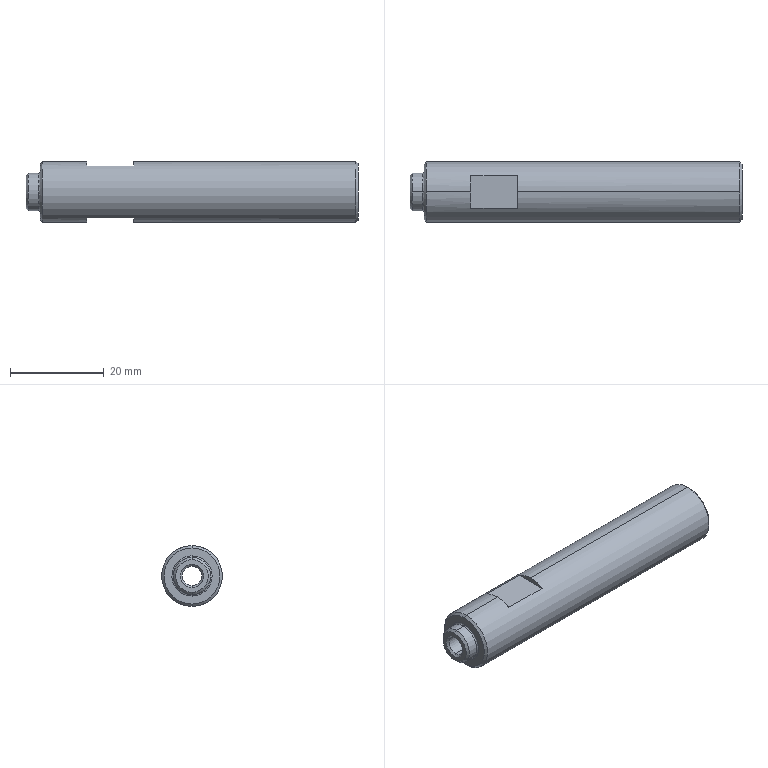Part | STEP file | sfppa13_68_f3_p8_m5_n5_sc10_2_03 | 1 solid | 27 faces | box 71 x 13 x 13 mm | volume 8114 mm3 | cone 10 | plane 9 | cylinder 6 | spline 2 | commonest cylinder face diameters 4.134 x2 8 x2 13 x2